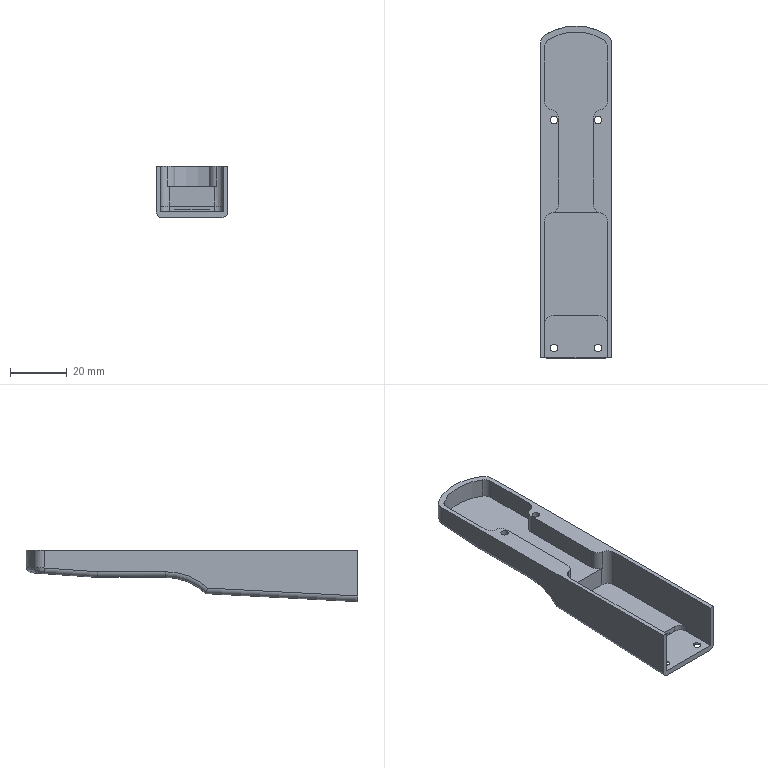Part | STEP file | ASND-0110-4216101100 | 1 solid | 71 faces | box 25 x 116.5 x 18 mm | volume 12649 mm3 | cylinder 35 | plane 23 | cone 8 | spline 3 | torus 2 | commonest cylinder face diameters 6 x12 4 x10 2.7 x8 8 x2 40 x2 36 x1